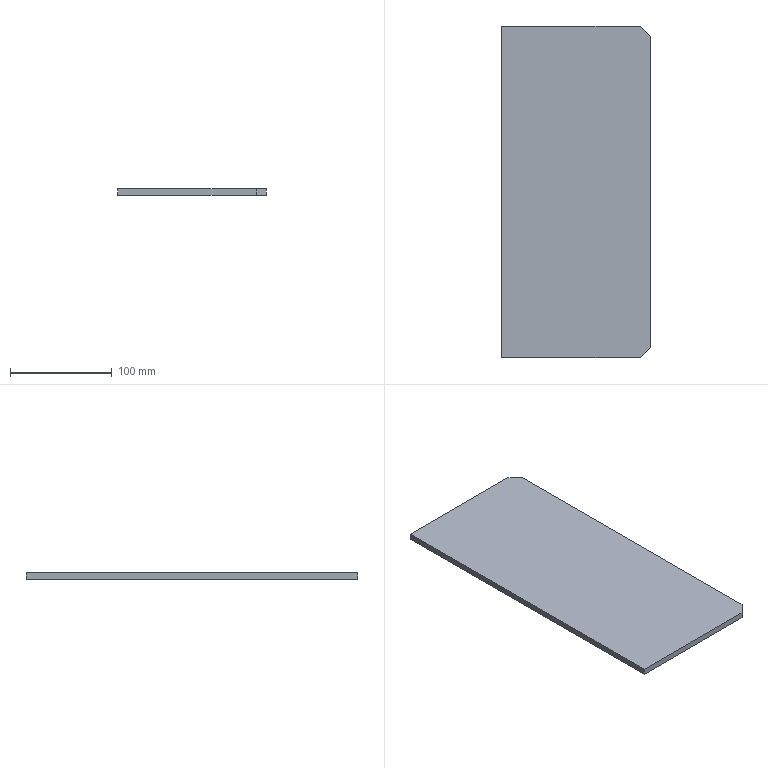Part | STEP file | 01-Rib plate 1 | 1 solid | 8 faces | box 146 x 325 x 6 mm | volume 284100 mm3 | plane 8
STEP:
#1=CARTESIAN_POINT('',(0.,0.,0.));
#2=DIRECTION('',(0.,0.,1.));
#3=DIRECTION('',(1.,0.,0.));
#4=AXIS2_PLACEMENT_3D('',#1,#2,#3);
#5=CARTESIAN_POINT('',(0.,0.,0.));
#6=VERTEX_POINT('',#5);
#7=CARTESIAN_POINT('',(0.,-325.,0.));
#8=VERTEX_POINT('',#7);
#9=CARTESIAN_POINT('',(0.,0.,0.));
#10=DIRECTION('',(0.,-1.,0.));
#11=VECTOR('',#10,1.);
#12=LINE('',#9,#11);
#13=CARTESIAN_POINT('',(0.,0.,6.));
#14=DIRECTION('',(1.,0.,0.));
#15=DIRECTION('',(0.,1.,0.));
#16=AXIS2_PLACEMENT_3D('',#13,#14,#15);
#17=PLANE('',#16);
#18=CARTESIAN_POINT('',(0.,-6.));
#19=DIRECTION('',(-1.,0.));
#20=VECTOR('',#19,1.);
#21=LINE('',#18,#20);
#22=(GEOMETRIC_REPRESENTATION_CONTEXT(2)PARAMETRIC_REPRESENTATION_CONTEXT()REPRESENTATION_CONTEXT('',''));
#23=DEFINITIONAL_REPRESENTATION('',(#21),#22);
#24=PCURVE('',#17,#23);
#25=CARTESIAN_POINT('',(0.,0.,0.));
#26=DIRECTION('',(0.,0.,1.));
#27=DIRECTION('',(1.,0.,0.));
#28=AXIS2_PLACEMENT_3D('',#25,#26,#27);
#29=PLANE('',#28);
#30=CARTESIAN_POINT('',(0.,0.));
#31=DIRECTION('',(0.,-1.));
#32=VECTOR('',#31,1.);
#33=LINE('',#30,#32);
#34=(GEOMETRIC_REPRESENTATION_CONTEXT(2)PARAMETRIC_REPRESENTATION_CONTEXT()REPRESENTATION_CONTEXT('',''));
#35=DEFINITIONAL_REPRESENTATION('',(#33),#34);
#36=PCURVE('',#29,#35);
#37=SURFACE_CURVE('',#12,(#24,#36),.PCURVE_S1.);
#38=EDGE_CURVE('',#6,#8,#37,.T.);
#39=ORIENTED_EDGE('',*,*,#38,.T.);
#40=CARTESIAN_POINT('',(0.,-325.,6.));
#41=VERTEX_POINT('',#40);
#42=CARTESIAN_POINT('',(0.,-325.,6.));
#43=DIRECTION('',(0.,0.,-1.));
#44=VECTOR('',#43,1.);
#45=LINE('',#42,#44);
#46=CARTESIAN_POINT('',(-325.,0.));
#47=DIRECTION('',(0.,-1.));
#48=VECTOR('',#47,1.);
#49=LINE('',#46,#48);
#50=(GEOMETRIC_REPRESENTATION_CONTEXT(2)PARAMETRIC_REPRESENTATION_CONTEXT()REPRESENTATION_CONTEXT('',''));
#51=DEFINITIONAL_REPRESENTATION('',(#49),#50);
#52=PCURVE('',#17,#51);
#53=CARTESIAN_POINT('',(0.,-325.,6.));
#54=DIRECTION('',(0.,1.,0.));
#55=DIRECTION('',(0.,0.,1.));
#56=AXIS2_PLACEMENT_3D('',#53,#54,#55);
#57=PLANE('',#56);
#58=CARTESIAN_POINT('',(0.,0.));
#59=DIRECTION('',(-1.,0.));
#60=VECTOR('',#59,1.);
#61=LINE('',#58,#60);
#62=(GEOMETRIC_REPRESENTATION_CONTEXT(2)PARAMETRIC_REPRESENTATION_CONTEXT()REPRESENTATION_CONTEXT('',''));
#63=DEFINITIONAL_REPRESENTATION('',(#61),#62);
#64=PCURVE('',#57,#63);
#65=SURFACE_CURVE('',#45,(#52,#64),.PCURVE_S1.);
#66=EDGE_CURVE('',#41,#8,#65,.T.);
#67=ORIENTED_EDGE('',*,*,#66,.F.);
#68=CARTESIAN_POINT('',(0.,0.,6.));
#69=VERTEX_POINT('',#68);
#70=CARTESIAN_POINT('',(0.,0.,6.));
#71=DIRECTION('',(0.,-1.,0.));
#72=VECTOR('',#71,1.);
#73=LINE('',#70,#72);
#74=CARTESIAN_POINT('',(0.,0.));
#75=DIRECTION('',(-1.,0.));
#76=VECTOR('',#75,1.);
#77=LINE('',#74,#76);
#78=(GEOMETRIC_REPRESENTATION_CONTEXT(2)PARAMETRIC_REPRESENTATION_CONTEXT()REPRESENTATION_CONTEXT('',''));
#79=DEFINITIONAL_REPRESENTATION('',(#77),#78);
#80=PCURVE('',#17,#79);
#81=CARTESIAN_POINT('',(0.,0.,6.));
#82=DIRECTION('',(0.,0.,1.));
#83=DIRECTION('',(1.,0.,0.));
#84=AXIS2_PLACEMENT_3D('',#81,#82,#83);
#85=PLANE('',#84);
#86=CARTESIAN_POINT('',(0.,0.));
#87=DIRECTION('',(0.,-1.));
#88=VECTOR('',#87,1.);
#89=LINE('',#86,#88);
#90=(GEOMETRIC_REPRESENTATION_CONTEXT(2)PARAMETRIC_REPRESENTATION_CONTEXT()REPRESENTATION_CONTEXT('',''));
#91=DEFINITIONAL_REPRESENTATION('',(#89),#90);
#92=PCURVE('',#85,#91);
#93=SURFACE_CURVE('',#73,(#80,#92),.PCURVE_S1.);
#94=EDGE_CURVE('',#69,#41,#93,.T.);
#95=ORIENTED_EDGE('',*,*,#94,.F.);
#96=CARTESIAN_POINT('',(0.,0.,6.));
#97=DIRECTION('',(0.,0.,-1.));
#98=VECTOR('',#97,1.);
#99=LINE('',#96,#98);
#100=CARTESIAN_POINT('',(0.,0.));
#101=DIRECTION('',(0.,-1.));
#102=VECTOR('',#101,1.);
#103=LINE('',#100,#102);
#104=(GEOMETRIC_REPRESENTATION_CONTEXT(2)PARAMETRIC_REPRESENTATION_CONTEXT()REPRESENTATION_CONTEXT('',''));
#105=DEFINITIONAL_REPRESENTATION('',(#103),#104);
#106=PCURVE('',#17,#105);
#107=CARTESIAN_POINT('',(0.,0.,6.));
#108=DIRECTION('',(0.,-1.,0.));
#109=DIRECTION('',(0.,0.,-1.));
#110=AXIS2_PLACEMENT_3D('',#107,#108,#109);
#111=PLANE('',#110);
#112=CARTESIAN_POINT('',(0.,0.));
#113=DIRECTION('',(1.,0.));
#114=VECTOR('',#113,1.);
#115=LINE('',#112,#114);
#116=(GEOMETRIC_REPRESENTATION_CONTEXT(2)PARAMETRIC_REPRESENTATION_CONTEXT()REPRESENTATION_CONTEXT('',''));
#117=DEFINITIONAL_REPRESENTATION('',(#115),#116);
#118=PCURVE('',#111,#117);
#119=SURFACE_CURVE('',#99,(#106,#118),.PCURVE_S1.);
#120=EDGE_CURVE('',#69,#6,#119,.T.);
#121=ORIENTED_EDGE('',*,*,#120,.T.);
#122=EDGE_LOOP('',(#39,#67,#95,#121));
#123=FACE_BOUND('',#122,.T.);
#124=ADVANCED_FACE('',(#123),#17,.F.);
#125=CARTESIAN_POINT('',(136.,-325.,0.));
#126=VERTEX_POINT('',#125);
#127=CARTESIAN_POINT('',(0.,-325.,0.));
#128=DIRECTION('',(1.,0.,0.));
#129=VECTOR('',#128,1.);
#130=LINE('',#127,#129);
#131=CARTESIAN_POINT('',(-6.,0.));
#132=DIRECTION('',(0.,1.));
#133=VECTOR('',#132,1.);
#134=LINE('',#131,#133);
#135=(GEOMETRIC_REPRESENTATION_CONTEXT(2)PARAMETRIC_REPRESENTATION_CONTEXT()REPRESENTATION_CONTEXT('',''));
#136=DEFINITIONAL_REPRESENTATION('',(#134),#135);
#137=PCURVE('',#57,#136);
#138=CARTESIAN_POINT('',(0.,-325.));
#139=DIRECTION('',(1.,0.));
#140=VECTOR('',#139,1.);
#141=LINE('',#138,#140);
#142=(GEOMETRIC_REPRESENTATION_CONTEXT(2)PARAMETRIC_REPRESENTATION_CONTEXT()REPRESENTATION_CONTEXT('',''));
#143=DEFINITIONAL_REPRESENTATION('',(#141),#142);
#144=PCURVE('',#29,#143);
#145=SURFACE_CURVE('',#130,(#137,#144),.PCURVE_S1.);
#146=EDGE_CURVE('',#8,#126,#145,.T.);
#147=ORIENTED_EDGE('',*,*,#146,.T.);
#148=CARTESIAN_POINT('',(136.,-325.,6.));
#149=VERTEX_POINT('',#148);
#150=CARTESIAN_POINT('',(136.,-325.,6.));
#151=DIRECTION('',(0.,0.,-1.));
#152=VECTOR('',#151,1.);
#153=LINE('',#150,#152);
#154=CARTESIAN_POINT('',(0.,136.));
#155=DIRECTION('',(-1.,0.));
#156=VECTOR('',#155,1.);
#157=LINE('',#154,#156);
#158=(GEOMETRIC_REPRESENTATION_CONTEXT(2)PARAMETRIC_REPRESENTATION_CONTEXT()REPRESENTATION_CONTEXT('',''));
#159=DEFINITIONAL_REPRESENTATION('',(#157),#158);
#160=PCURVE('',#57,#159);
#161=CARTESIAN_POINT('',(146.,-315.,6.));
#162=DIRECTION('',(-0.7071,0.7071,0.));
#163=DIRECTION('',(-0.7071,-0.7071,0.));
#164=AXIS2_PLACEMENT_3D('',#161,#162,#163);
#165=PLANE('',#164);
#166=CARTESIAN_POINT('',(14.142,0.));
#167=DIRECTION('',(0.,-1.));
#168=VECTOR('',#167,1.);
#169=LINE('',#166,#168);
#170=(GEOMETRIC_REPRESENTATION_CONTEXT(2)PARAMETRIC_REPRESENTATION_CONTEXT()REPRESENTATION_CONTEXT('',''));
#171=DEFINITIONAL_REPRESENTATION('',(#169),#170);
#172=PCURVE('',#165,#171);
#173=SURFACE_CURVE('',#153,(#160,#172),.PCURVE_S1.);
#174=EDGE_CURVE('',#149,#126,#173,.T.);
#175=ORIENTED_EDGE('',*,*,#174,.F.);
#176=CARTESIAN_POINT('',(0.,-325.,6.));
#177=DIRECTION('',(1.,0.,0.));
#178=VECTOR('',#177,1.);
#179=LINE('',#176,#178);
#180=CARTESIAN_POINT('',(0.,0.));
#181=DIRECTION('',(0.,1.));
#182=VECTOR('',#181,1.);
#183=LINE('',#180,#182);
#184=(GEOMETRIC_REPRESENTATION_CONTEXT(2)PARAMETRIC_REPRESENTATION_CONTEXT()REPRESENTATION_CONTEXT('',''));
#185=DEFINITIONAL_REPRESENTATION('',(#183),#184);
#186=PCURVE('',#57,#185);
#187=CARTESIAN_POINT('',(0.,-325.));
#188=DIRECTION('',(1.,0.));
#189=VECTOR('',#188,1.);
#190=LINE('',#187,#189);
#191=(GEOMETRIC_REPRESENTATION_CONTEXT(2)PARAMETRIC_REPRESENTATION_CONTEXT()REPRESENTATION_CONTEXT('',''));
#192=DEFINITIONAL_REPRESENTATION('',(#190),#191);
#193=PCURVE('',#85,#192);
#194=SURFACE_CURVE('',#179,(#186,#193),.PCURVE_S1.);
#195=EDGE_CURVE('',#41,#149,#194,.T.);
#196=ORIENTED_EDGE('',*,*,#195,.F.);
#197=ORIENTED_EDGE('',*,*,#66,.T.);
#198=EDGE_LOOP('',(#147,#175,#196,#197));
#199=FACE_BOUND('',#198,.T.);
#200=ADVANCED_FACE('',(#199),#57,.F.);
#201=CARTESIAN_POINT('',(146.,-315.,0.));
#202=VERTEX_POINT('',#201);
#203=CARTESIAN_POINT('',(146.,-315.,0.));
#204=DIRECTION('',(0.7071,0.7071,0.));
#205=VECTOR('',#204,1.);
#206=LINE('',#203,#205);
#207=CARTESIAN_POINT('',(0.,-6.));
#208=DIRECTION('',(-1.,0.));
#209=VECTOR('',#208,1.);
#210=LINE('',#207,#209);
#211=(GEOMETRIC_REPRESENTATION_CONTEXT(2)PARAMETRIC_REPRESENTATION_CONTEXT()REPRESENTATION_CONTEXT('',''));
#212=DEFINITIONAL_REPRESENTATION('',(#210),#211);
#213=PCURVE('',#165,#212);
#214=CARTESIAN_POINT('',(146.,-315.));
#215=DIRECTION('',(0.7071,0.7071));
#216=VECTOR('',#215,1.);
#217=LINE('',#214,#216);
#218=(GEOMETRIC_REPRESENTATION_CONTEXT(2)PARAMETRIC_REPRESENTATION_CONTEXT()REPRESENTATION_CONTEXT('',''));
#219=DEFINITIONAL_REPRESENTATION('',(#217),#218);
#220=PCURVE('',#29,#219);
#221=SURFACE_CURVE('',#206,(#213,#220),.PCURVE_S1.);
#222=EDGE_CURVE('',#126,#202,#221,.T.);
#223=ORIENTED_EDGE('',*,*,#222,.T.);
#224=CARTESIAN_POINT('',(146.,-315.,6.));
#225=VERTEX_POINT('',#224);
#226=CARTESIAN_POINT('',(146.,-315.,6.));
#227=DIRECTION('',(0.,0.,-1.));
#228=VECTOR('',#227,1.);
#229=LINE('',#226,#228);
#230=CARTESIAN_POINT('',(0.,0.));
#231=DIRECTION('',(0.,-1.));
#232=VECTOR('',#231,1.);
#233=LINE('',#230,#232);
#234=(GEOMETRIC_REPRESENTATION_CONTEXT(2)PARAMETRIC_REPRESENTATION_CONTEXT()REPRESENTATION_CONTEXT('',''));
#235=DEFINITIONAL_REPRESENTATION('',(#233),#234);
#236=PCURVE('',#165,#235);
#237=CARTESIAN_POINT('',(146.,-10.,6.));
#238=DIRECTION('',(-1.,0.,0.));
#239=DIRECTION('',(0.,-1.,0.));
#240=AXIS2_PLACEMENT_3D('',#237,#238,#239);
#241=PLANE('',#240);
#242=CARTESIAN_POINT('',(305.,0.));
#243=DIRECTION('',(0.,-1.));
#244=VECTOR('',#243,1.);
#245=LINE('',#242,#244);
#246=(GEOMETRIC_REPRESENTATION_CONTEXT(2)PARAMETRIC_REPRESENTATION_CONTEXT()REPRESENTATION_CONTEXT('',''));
#247=DEFINITIONAL_REPRESENTATION('',(#245),#246);
#248=PCURVE('',#241,#247);
#249=SURFACE_CURVE('',#229,(#236,#248),.PCURVE_S1.);
#250=EDGE_CURVE('',#225,#202,#249,.T.);
#251=ORIENTED_EDGE('',*,*,#250,.F.);
#252=CARTESIAN_POINT('',(146.,-315.,6.));
#253=DIRECTION('',(0.7071,0.7071,0.));
#254=VECTOR('',#253,1.);
#255=LINE('',#252,#254);
#256=CARTESIAN_POINT('',(0.,0.));
#257=DIRECTION('',(-1.,0.));
#258=VECTOR('',#257,1.);
#259=LINE('',#256,#258);
#260=(GEOMETRIC_REPRESENTATION_CONTEXT(2)PARAMETRIC_REPRESENTATION_CONTEXT()REPRESENTATION_CONTEXT('',''));
#261=DEFINITIONAL_REPRESENTATION('',(#259),#260);
#262=PCURVE('',#165,#261);
#263=CARTESIAN_POINT('',(146.,-315.));
#264=DIRECTION('',(0.7071,0.7071));
#265=VECTOR('',#264,1.);
#266=LINE('',#263,#265);
#267=(GEOMETRIC_REPRESENTATION_CONTEXT(2)PARAMETRIC_REPRESENTATION_CONTEXT()REPRESENTATION_CONTEXT('',''));
#268=DEFINITIONAL_REPRESENTATION('',(#266),#267);
#269=PCURVE('',#85,#268);
#270=SURFACE_CURVE('',#255,(#262,#269),.PCURVE_S1.);
#271=EDGE_CURVE('',#149,#225,#270,.T.);
#272=ORIENTED_EDGE('',*,*,#271,.F.);
#273=ORIENTED_EDGE('',*,*,#174,.T.);
#274=EDGE_LOOP('',(#223,#251,#272,#273));
#275=FACE_BOUND('',#274,.T.);
#276=ADVANCED_FACE('',(#275),#165,.F.);
#277=CARTESIAN_POINT('',(146.,-10.,0.));
#278=VERTEX_POINT('',#277);
#279=CARTESIAN_POINT('',(146.,-10.,0.));
#280=DIRECTION('',(0.,1.,0.));
#281=VECTOR('',#280,1.);
#282=LINE('',#279,#281);
#283=CARTESIAN_POINT('',(0.,-6.));
#284=DIRECTION('',(-1.,0.));
#285=VECTOR('',#284,1.);
#286=LINE('',#283,#285);
#287=(GEOMETRIC_REPRESENTATION_CONTEXT(2)PARAMETRIC_REPRESENTATION_CONTEXT()REPRESENTATION_CONTEXT('',''));
#288=DEFINITIONAL_REPRESENTATION('',(#286),#287);
#289=PCURVE('',#241,#288);
#290=CARTESIAN_POINT('',(146.,-10.));
#291=DIRECTION('',(0.,1.));
#292=VECTOR('',#291,1.);
#293=LINE('',#290,#292);
#294=(GEOMETRIC_REPRESENTATION_CONTEXT(2)PARAMETRIC_REPRESENTATION_CONTEXT()REPRESENTATION_CONTEXT('',''));
#295=DEFINITIONAL_REPRESENTATION('',(#293),#294);
#296=PCURVE('',#29,#295);
#297=SURFACE_CURVE('',#282,(#289,#296),.PCURVE_S1.);
#298=EDGE_CURVE('',#202,#278,#297,.T.);
#299=ORIENTED_EDGE('',*,*,#298,.T.);
#300=CARTESIAN_POINT('',(146.,-10.,6.));
#301=VERTEX_POINT('',#300);
#302=CARTESIAN_POINT('',(146.,-10.,6.));
#303=DIRECTION('',(0.,0.,-1.));
#304=VECTOR('',#303,1.);
#305=LINE('',#302,#304);
#306=CARTESIAN_POINT('',(0.,0.));
#307=DIRECTION('',(0.,-1.));
#308=VECTOR('',#307,1.);
#309=LINE('',#306,#308);
#310=(GEOMETRIC_REPRESENTATION_CONTEXT(2)PARAMETRIC_REPRESENTATION_CONTEXT()REPRESENTATION_CONTEXT('',''));
#311=DEFINITIONAL_REPRESENTATION('',(#309),#310);
#312=PCURVE('',#241,#311);
#313=CARTESIAN_POINT('',(136.,0.,6.));
#314=DIRECTION('',(-0.7071,-0.7071,0.));
#315=DIRECTION('',(0.7071,-0.7071,0.));
#316=AXIS2_PLACEMENT_3D('',#313,#314,#315);
#317=PLANE('',#316);
#318=CARTESIAN_POINT('',(14.142,0.));
#319=DIRECTION('',(0.,-1.));
#320=VECTOR('',#319,1.);
#321=LINE('',#318,#320);
#322=(GEOMETRIC_REPRESENTATION_CONTEXT(2)PARAMETRIC_REPRESENTATION_CONTEXT()REPRESENTATION_CONTEXT('',''));
#323=DEFINITIONAL_REPRESENTATION('',(#321),#322);
#324=PCURVE('',#317,#323);
#325=SURFACE_CURVE('',#305,(#312,#324),.PCURVE_S1.);
#326=EDGE_CURVE('',#301,#278,#325,.T.);
#327=ORIENTED_EDGE('',*,*,#326,.F.);
#328=CARTESIAN_POINT('',(146.,-10.,6.));
#329=DIRECTION('',(0.,1.,0.));
#330=VECTOR('',#329,1.);
#331=LINE('',#328,#330);
#332=CARTESIAN_POINT('',(0.,0.));
#333=DIRECTION('',(-1.,0.));
#334=VECTOR('',#333,1.);
#335=LINE('',#332,#334);
#336=(GEOMETRIC_REPRESENTATION_CONTEXT(2)PARAMETRIC_REPRESENTATION_CONTEXT()REPRESENTATION_CONTEXT('',''));
#337=DEFINITIONAL_REPRESENTATION('',(#335),#336);
#338=PCURVE('',#241,#337);
#339=CARTESIAN_POINT('',(146.,-10.));
#340=DIRECTION('',(0.,1.));
#341=VECTOR('',#340,1.);
#342=LINE('',#339,#341);
#343=(GEOMETRIC_REPRESENTATION_CONTEXT(2)PARAMETRIC_REPRESENTATION_CONTEXT()REPRESENTATION_CONTEXT('',''));
#344=DEFINITIONAL_REPRESENTATION('',(#342),#343);
#345=PCURVE('',#85,#344);
#346=SURFACE_CURVE('',#331,(#338,#345),.PCURVE_S1.);
#347=EDGE_CURVE('',#225,#301,#346,.T.);
#348=ORIENTED_EDGE('',*,*,#347,.F.);
#349=ORIENTED_EDGE('',*,*,#250,.T.);
#350=EDGE_LOOP('',(#299,#327,#348,#349));
#351=FACE_BOUND('',#350,.T.);
#352=ADVANCED_FACE('',(#351),#241,.F.);
#353=CARTESIAN_POINT('',(136.,0.,0.));
#354=VERTEX_POINT('',#353);
#355=CARTESIAN_POINT('',(136.,0.,0.));
#356=DIRECTION('',(-0.7071,0.7071,0.));
#357=VECTOR('',#356,1.);
#358=LINE('',#355,#357);
#359=CARTESIAN_POINT('',(0.,-6.));
#360=DIRECTION('',(-1.,0.));
#361=VECTOR('',#360,1.);
#362=LINE('',#359,#361);
#363=(GEOMETRIC_REPRESENTATION_CONTEXT(2)PARAMETRIC_REPRESENTATION_CONTEXT()REPRESENTATION_CONTEXT('',''));
#364=DEFINITIONAL_REPRESENTATION('',(#362),#363);
#365=PCURVE('',#317,#364);
#366=CARTESIAN_POINT('',(136.,0.));
#367=DIRECTION('',(-0.7071,0.7071));
#368=VECTOR('',#367,1.);
#369=LINE('',#366,#368);
#370=(GEOMETRIC_REPRESENTATION_CONTEXT(2)PARAMETRIC_REPRESENTATION_CONTEXT()REPRESENTATION_CONTEXT('',''));
#371=DEFINITIONAL_REPRESENTATION('',(#369),#370);
#372=PCURVE('',#29,#371);
#373=SURFACE_CURVE('',#358,(#365,#372),.PCURVE_S1.);
#374=EDGE_CURVE('',#278,#354,#373,.T.);
#375=ORIENTED_EDGE('',*,*,#374,.T.);
#376=CARTESIAN_POINT('',(136.,0.,6.));
#377=VERTEX_POINT('',#376);
#378=CARTESIAN_POINT('',(136.,0.,6.));
#379=DIRECTION('',(0.,0.,-1.));
#380=VECTOR('',#379,1.);
#381=LINE('',#378,#380);
#382=CARTESIAN_POINT('',(0.,0.));
#383=DIRECTION('',(0.,-1.));
#384=VECTOR('',#383,1.);
#385=LINE('',#382,#384);
#386=(GEOMETRIC_REPRESENTATION_CONTEXT(2)PARAMETRIC_REPRESENTATION_CONTEXT()REPRESENTATION_CONTEXT('',''));
#387=DEFINITIONAL_REPRESENTATION('',(#385),#386);
#388=PCURVE('',#317,#387);
#389=CARTESIAN_POINT('',(0.,136.));
#390=DIRECTION('',(1.,0.));
#391=VECTOR('',#390,1.);
#392=LINE('',#389,#391);
#393=(GEOMETRIC_REPRESENTATION_CONTEXT(2)PARAMETRIC_REPRESENTATION_CONTEXT()REPRESENTATION_CONTEXT('',''));
#394=DEFINITIONAL_REPRESENTATION('',(#392),#393);
#395=PCURVE('',#111,#394);
#396=SURFACE_CURVE('',#381,(#388,#395),.PCURVE_S1.);
#397=EDGE_CURVE('',#377,#354,#396,.T.);
#398=ORIENTED_EDGE('',*,*,#397,.F.);
#399=CARTESIAN_POINT('',(136.,0.,6.));
#400=DIRECTION('',(-0.7071,0.7071,0.));
#401=VECTOR('',#400,1.);
#402=LINE('',#399,#401);
#403=CARTESIAN_POINT('',(0.,0.));
#404=DIRECTION('',(-1.,0.));
#405=VECTOR('',#404,1.);
#406=LINE('',#403,#405);
#407=(GEOMETRIC_REPRESENTATION_CONTEXT(2)PARAMETRIC_REPRESENTATION_CONTEXT()REPRESENTATION_CONTEXT('',''));
#408=DEFINITIONAL_REPRESENTATION('',(#406),#407);
#409=PCURVE('',#317,#408);
#410=CARTESIAN_POINT('',(136.,0.));
#411=DIRECTION('',(-0.7071,0.7071));
#412=VECTOR('',#411,1.);
#413=LINE('',#410,#412);
#414=(GEOMETRIC_REPRESENTATION_CONTEXT(2)PARAMETRIC_REPRESENTATION_CONTEXT()REPRESENTATION_CONTEXT('',''));
#415=DEFINITIONAL_REPRESENTATION('',(#413),#414);
#416=PCURVE('',#85,#415);
#417=SURFACE_CURVE('',#402,(#409,#416),.PCURVE_S1.);
#418=EDGE_CURVE('',#301,#377,#417,.T.);
#419=ORIENTED_EDGE('',*,*,#418,.F.);
#420=ORIENTED_EDGE('',*,*,#326,.T.);
#421=EDGE_LOOP('',(#375,#398,#419,#420));
#422=FACE_BOUND('',#421,.T.);
#423=ADVANCED_FACE('',(#422),#317,.F.);
#424=CARTESIAN_POINT('',(0.,0.,0.));
#425=DIRECTION('',(-1.,0.,0.));
#426=VECTOR('',#425,1.);
#427=LINE('',#424,#426);
#428=CARTESIAN_POINT('',(6.,0.));
#429=DIRECTION('',(0.,-1.));
#430=VECTOR('',#429,1.);
#431=LINE('',#428,#430);
#432=(GEOMETRIC_REPRESENTATION_CONTEXT(2)PARAMETRIC_REPRESENTATION_CONTEXT()REPRESENTATION_CONTEXT('',''));
#433=DEFINITIONAL_REPRESENTATION('',(#431),#432);
#434=PCURVE('',#111,#433);
#435=CARTESIAN_POINT('',(0.,0.));
#436=DIRECTION('',(-1.,0.));
#437=VECTOR('',#436,1.);
#438=LINE('',#435,#437);
#439=(GEOMETRIC_REPRESENTATION_CONTEXT(2)PARAMETRIC_REPRESENTATION_CONTEXT()REPRESENTATION_CONTEXT('',''));
#440=DEFINITIONAL_REPRESENTATION('',(#438),#439);
#441=PCURVE('',#29,#440);
#442=SURFACE_CURVE('',#427,(#434,#441),.PCURVE_S1.);
#443=EDGE_CURVE('',#354,#6,#442,.T.);
#444=ORIENTED_EDGE('',*,*,#443,.T.);
#445=ORIENTED_EDGE('',*,*,#120,.F.);
#446=CARTESIAN_POINT('',(0.,0.,6.));
#447=DIRECTION('',(-1.,0.,0.));
#448=VECTOR('',#447,1.);
#449=LINE('',#446,#448);
#450=CARTESIAN_POINT('',(0.,0.));
#451=DIRECTION('',(0.,-1.));
#452=VECTOR('',#451,1.);
#453=LINE('',#450,#452);
#454=(GEOMETRIC_REPRESENTATION_CONTEXT(2)PARAMETRIC_REPRESENTATION_CONTEXT()REPRESENTATION_CONTEXT('',''));
#455=DEFINITIONAL_REPRESENTATION('',(#453),#454);
#456=PCURVE('',#111,#455);
#457=CARTESIAN_POINT('',(0.,0.));
#458=DIRECTION('',(-1.,0.));
#459=VECTOR('',#458,1.);
#460=LINE('',#457,#459);
#461=(GEOMETRIC_REPRESENTATION_CONTEXT(2)PARAMETRIC_REPRESENTATION_CONTEXT()REPRESENTATION_CONTEXT('',''));
#462=DEFINITIONAL_REPRESENTATION('',(#460),#461);
#463=PCURVE('',#85,#462);
#464=SURFACE_CURVE('',#449,(#456,#463),.PCURVE_S1.);
#465=EDGE_CURVE('',#377,#69,#464,.T.);
#466=ORIENTED_EDGE('',*,*,#465,.F.);
#467=ORIENTED_EDGE('',*,*,#397,.T.);
#468=EDGE_LOOP('',(#444,#445,#466,#467));
#469=FACE_BOUND('',#468,.T.);
#470=ADVANCED_FACE('',(#469),#111,.F.);
#471=ORIENTED_EDGE('',*,*,#94,.T.);
#472=ORIENTED_EDGE('',*,*,#195,.T.);
#473=ORIENTED_EDGE('',*,*,#271,.T.);
#474=ORIENTED_EDGE('',*,*,#347,.T.);
#475=ORIENTED_EDGE('',*,*,#418,.T.);
#476=ORIENTED_EDGE('',*,*,#465,.T.);
#477=EDGE_LOOP('',(#471,#472,#473,#474,#475,#476));
#478=FACE_BOUND('',#477,.T.);
#479=ADVANCED_FACE('',(#478),#85,.T.);
#480=ORIENTED_EDGE('',*,*,#38,.F.);
#481=ORIENTED_EDGE('',*,*,#443,.F.);
#482=ORIENTED_EDGE('',*,*,#374,.F.);
#483=ORIENTED_EDGE('',*,*,#298,.F.);
#484=ORIENTED_EDGE('',*,*,#222,.F.);
#485=ORIENTED_EDGE('',*,*,#146,.F.);
#486=EDGE_LOOP('',(#480,#481,#482,#483,#484,#485));
#487=FACE_BOUND('',#486,.T.);
#488=ADVANCED_FACE('',(#487),#29,.F.);
#489=CLOSED_SHELL('',(#124,#200,#276,#352,#423,#470,#479,#488));
#490=MANIFOLD_SOLID_BREP('',#489);
#491=(LENGTH_UNIT()NAMED_UNIT(*)SI_UNIT(.MILLI.,.METRE.));
#492=UNCERTAINTY_MEASURE_WITH_UNIT(LENGTH_MEASURE(0.0000001),#491,'','');
#493=(NAMED_UNIT(*)PLANE_ANGLE_UNIT()SI_UNIT($,.RADIAN.));
#494=(NAMED_UNIT(*)SI_UNIT($,.STERADIAN.)SOLID_ANGLE_UNIT());
#495=(GEOMETRIC_REPRESENTATION_CONTEXT(3)GLOBAL_UNCERTAINTY_ASSIGNED_CONTEXT((#492))GLOBAL_UNIT_ASSIGNED_CONTEXT((#491,#493,#494))REPRESENTATION_CONTEXT('',''));
#496=ADVANCED_BREP_SHAPE_REPRESENTATION('',(#4,#490),#495);